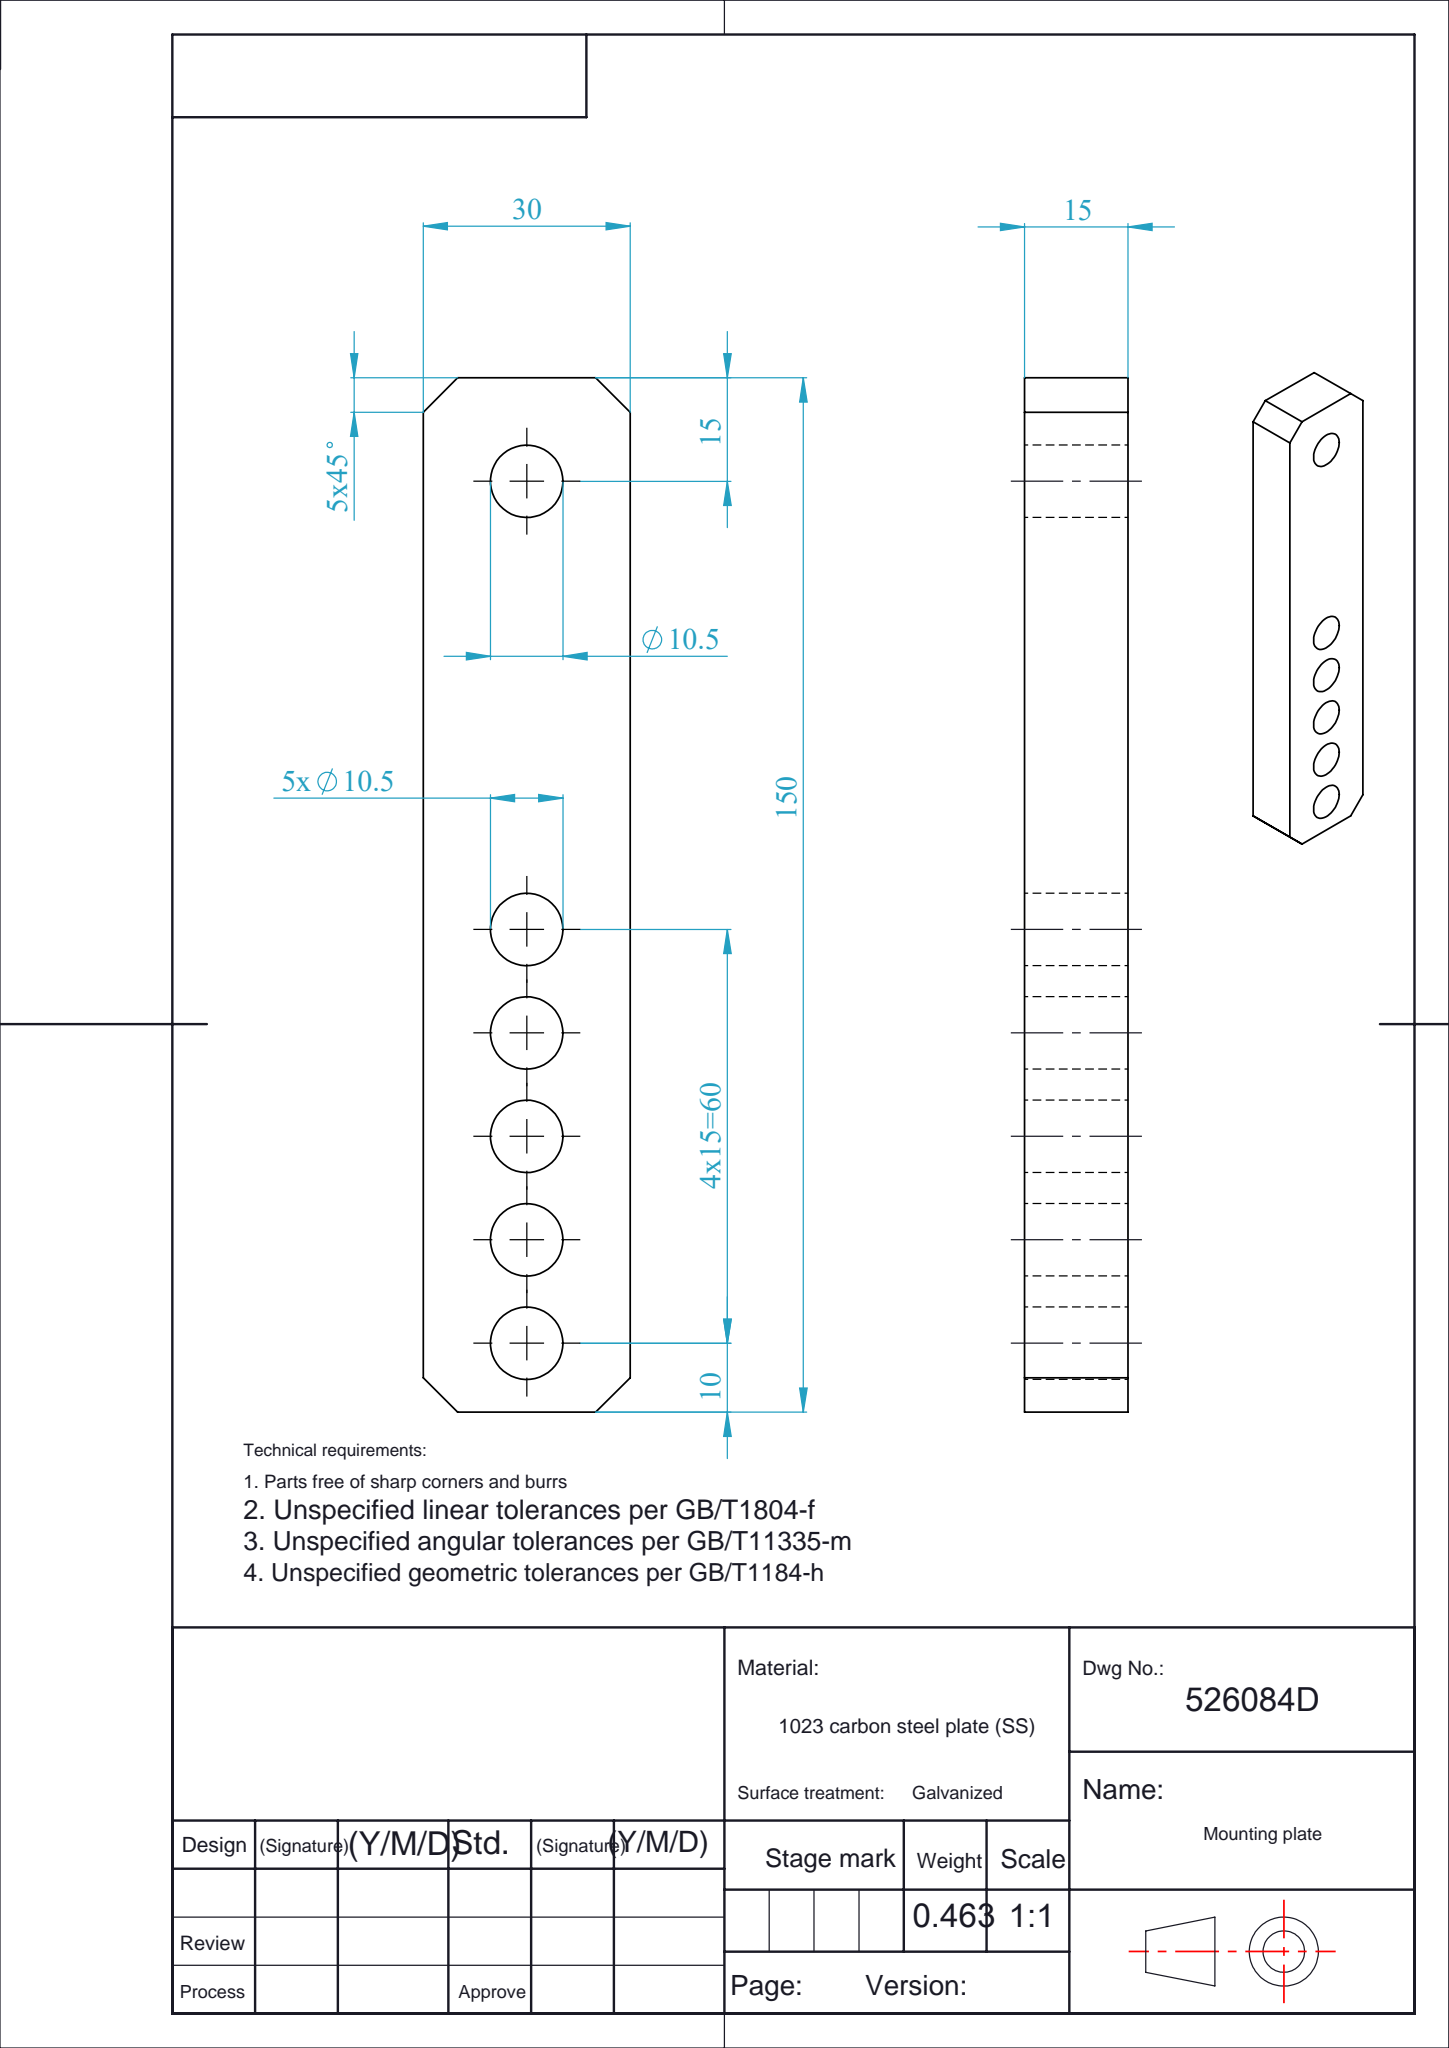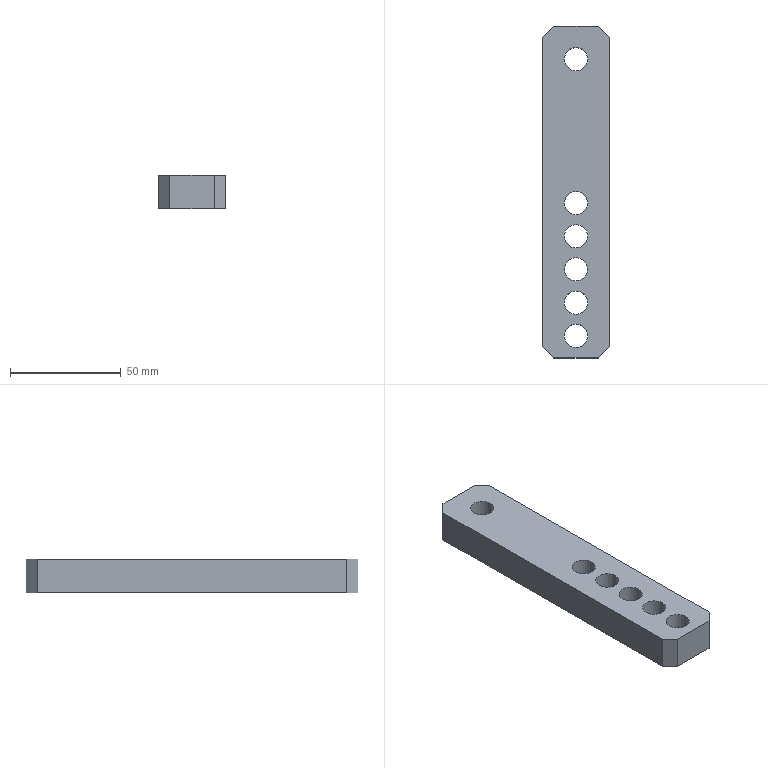Part | SolidWorks | features Chamfer 1, Extrusion 1, ICE 1 | 1 solid | 22 faces | box 30 x 150 x 15 mm | volume 58957 mm3 | cylinder 12 | plane 10 | commonest cylinder face diameters 10.5 x12
STEP:
#1=CARTESIAN_POINT('',(-5.25,60.,0.));
#2=VERTEX_POINT('',#1);
#3=CARTESIAN_POINT('',(5.25,60.,0.));
#4=VERTEX_POINT('',#3);
#5=CARTESIAN_POINT('',(0.,60.,0.));
#6=DIRECTION('',(0.,0.,1.));
#7=DIRECTION('',(1.,0.,0.));
#8=AXIS2_PLACEMENT_3D('',#5,#6,#7);
#9=CIRCLE('',#8,5.25);
#10=EDGE_CURVE('',#2,#4,#9,.T.);
#11=ORIENTED_EDGE('',*,*,#10,.F.);
#12=CARTESIAN_POINT('',(-5.25,60.,15.));
#13=VERTEX_POINT('',#12);
#14=CARTESIAN_POINT('',(-5.25,60.,-28.));
#15=DIRECTION('',(0.,0.,1.));
#16=VECTOR('',#15,1000.);
#17=LINE('',#14,#16);
#18=EDGE_CURVE('',#2,#13,#17,.T.);
#19=ORIENTED_EDGE('',*,*,#18,.T.);
#20=CARTESIAN_POINT('',(5.25,60.,15.));
#21=VERTEX_POINT('',#20);
#22=CARTESIAN_POINT('',(0.,60.,15.));
#23=DIRECTION('',(0.,0.,1.));
#24=DIRECTION('',(1.,0.,0.));
#25=AXIS2_PLACEMENT_3D('',#22,#23,#24);
#26=CIRCLE('',#25,5.25);
#27=EDGE_CURVE('',#13,#21,#26,.T.);
#28=ORIENTED_EDGE('',*,*,#27,.T.);
#29=CARTESIAN_POINT('',(5.25,60.,-28.));
#30=DIRECTION('',(0.,0.,1.));
#31=VECTOR('',#30,1000.);
#32=LINE('',#29,#31);
#33=EDGE_CURVE('',#4,#21,#32,.T.);
#34=ORIENTED_EDGE('',*,*,#33,.F.);
#35=EDGE_LOOP('',(#11,#19,#28,#34));
#36=FACE_OUTER_BOUND('',#35,.T.);
#37=CARTESIAN_POINT('',(0.,60.,-28.));
#38=DIRECTION('',(0.,0.,1.));
#39=DIRECTION('',(1.,0.,0.));
#40=AXIS2_PLACEMENT_3D('',#37,#38,#39);
#41=CYLINDRICAL_SURFACE('',#40,5.25);
#42=ADVANCED_FACE('',(#36),#41,.F.);
#43=CARTESIAN_POINT('',(-5.25,-5.,0.));
#44=VERTEX_POINT('',#43);
#45=CARTESIAN_POINT('',(5.25,-5.,0.));
#46=VERTEX_POINT('',#45);
#47=CARTESIAN_POINT('',(0.,-5.,0.));
#48=DIRECTION('',(0.,0.,1.));
#49=DIRECTION('',(1.,0.,0.));
#50=AXIS2_PLACEMENT_3D('',#47,#48,#49);
#51=CIRCLE('',#50,5.25);
#52=EDGE_CURVE('',#44,#46,#51,.T.);
#53=ORIENTED_EDGE('',*,*,#52,.F.);
#54=CARTESIAN_POINT('',(-5.25,-5.,15.));
#55=VERTEX_POINT('',#54);
#56=CARTESIAN_POINT('',(-5.25,-5.,-28.));
#57=DIRECTION('',(0.,0.,1.));
#58=VECTOR('',#57,1000.);
#59=LINE('',#56,#58);
#60=EDGE_CURVE('',#44,#55,#59,.T.);
#61=ORIENTED_EDGE('',*,*,#60,.T.);
#62=CARTESIAN_POINT('',(5.25,-5.,15.));
#63=VERTEX_POINT('',#62);
#64=CARTESIAN_POINT('',(0.,-5.,15.));
#65=DIRECTION('',(0.,0.,1.));
#66=DIRECTION('',(1.,0.,0.));
#67=AXIS2_PLACEMENT_3D('',#64,#65,#66);
#68=CIRCLE('',#67,5.25);
#69=EDGE_CURVE('',#55,#63,#68,.T.);
#70=ORIENTED_EDGE('',*,*,#69,.T.);
#71=CARTESIAN_POINT('',(5.25,-5.,-28.));
#72=DIRECTION('',(0.,0.,1.));
#73=VECTOR('',#72,1000.);
#74=LINE('',#71,#73);
#75=EDGE_CURVE('',#46,#63,#74,.T.);
#76=ORIENTED_EDGE('',*,*,#75,.F.);
#77=EDGE_LOOP('',(#53,#61,#70,#76));
#78=FACE_OUTER_BOUND('',#77,.T.);
#79=CARTESIAN_POINT('',(0.,-5.,-28.));
#80=DIRECTION('',(0.,0.,1.));
#81=DIRECTION('',(1.,0.,0.));
#82=AXIS2_PLACEMENT_3D('',#79,#80,#81);
#83=CYLINDRICAL_SURFACE('',#82,5.25);
#84=ADVANCED_FACE('',(#78),#83,.F.);
#85=CARTESIAN_POINT('',(-5.25,-20.,0.));
#86=VERTEX_POINT('',#85);
#87=CARTESIAN_POINT('',(5.25,-20.,0.));
#88=VERTEX_POINT('',#87);
#89=CARTESIAN_POINT('',(0.,-20.,0.));
#90=DIRECTION('',(0.,0.,1.));
#91=DIRECTION('',(1.,0.,0.));
#92=AXIS2_PLACEMENT_3D('',#89,#90,#91);
#93=CIRCLE('',#92,5.25);
#94=EDGE_CURVE('',#86,#88,#93,.T.);
#95=ORIENTED_EDGE('',*,*,#94,.F.);
#96=CARTESIAN_POINT('',(-5.25,-20.,15.));
#97=VERTEX_POINT('',#96);
#98=CARTESIAN_POINT('',(-5.25,-20.,-28.));
#99=DIRECTION('',(0.,0.,1.));
#100=VECTOR('',#99,1000.);
#101=LINE('',#98,#100);
#102=EDGE_CURVE('',#86,#97,#101,.T.);
#103=ORIENTED_EDGE('',*,*,#102,.T.);
#104=CARTESIAN_POINT('',(5.25,-20.,15.));
#105=VERTEX_POINT('',#104);
#106=CARTESIAN_POINT('',(0.,-20.,15.));
#107=DIRECTION('',(0.,0.,1.));
#108=DIRECTION('',(1.,0.,0.));
#109=AXIS2_PLACEMENT_3D('',#106,#107,#108);
#110=CIRCLE('',#109,5.25);
#111=EDGE_CURVE('',#97,#105,#110,.T.);
#112=ORIENTED_EDGE('',*,*,#111,.T.);
#113=CARTESIAN_POINT('',(5.25,-20.,-28.));
#114=DIRECTION('',(0.,0.,1.));
#115=VECTOR('',#114,1000.);
#116=LINE('',#113,#115);
#117=EDGE_CURVE('',#88,#105,#116,.T.);
#118=ORIENTED_EDGE('',*,*,#117,.F.);
#119=EDGE_LOOP('',(#95,#103,#112,#118));
#120=FACE_OUTER_BOUND('',#119,.T.);
#121=CARTESIAN_POINT('',(0.,-20.,-28.));
#122=DIRECTION('',(0.,0.,1.));
#123=DIRECTION('',(1.,0.,0.));
#124=AXIS2_PLACEMENT_3D('',#121,#122,#123);
#125=CYLINDRICAL_SURFACE('',#124,5.25);
#126=ADVANCED_FACE('',(#120),#125,.F.);
#127=CARTESIAN_POINT('',(-5.25,-35.,0.));
#128=VERTEX_POINT('',#127);
#129=CARTESIAN_POINT('',(5.25,-35.,0.));
#130=VERTEX_POINT('',#129);
#131=CARTESIAN_POINT('',(0.,-35.,0.));
#132=DIRECTION('',(0.,0.,1.));
#133=DIRECTION('',(1.,0.,0.));
#134=AXIS2_PLACEMENT_3D('',#131,#132,#133);
#135=CIRCLE('',#134,5.25);
#136=EDGE_CURVE('',#128,#130,#135,.T.);
#137=ORIENTED_EDGE('',*,*,#136,.F.);
#138=CARTESIAN_POINT('',(-5.25,-35.,15.));
#139=VERTEX_POINT('',#138);
#140=CARTESIAN_POINT('',(-5.25,-35.,-28.));
#141=DIRECTION('',(0.,0.,1.));
#142=VECTOR('',#141,1000.);
#143=LINE('',#140,#142);
#144=EDGE_CURVE('',#128,#139,#143,.T.);
#145=ORIENTED_EDGE('',*,*,#144,.T.);
#146=CARTESIAN_POINT('',(5.25,-35.,15.));
#147=VERTEX_POINT('',#146);
#148=CARTESIAN_POINT('',(0.,-35.,15.));
#149=DIRECTION('',(0.,0.,1.));
#150=DIRECTION('',(1.,0.,0.));
#151=AXIS2_PLACEMENT_3D('',#148,#149,#150);
#152=CIRCLE('',#151,5.25);
#153=EDGE_CURVE('',#139,#147,#152,.T.);
#154=ORIENTED_EDGE('',*,*,#153,.T.);
#155=CARTESIAN_POINT('',(5.25,-35.,-28.));
#156=DIRECTION('',(0.,0.,1.));
#157=VECTOR('',#156,1000.);
#158=LINE('',#155,#157);
#159=EDGE_CURVE('',#130,#147,#158,.T.);
#160=ORIENTED_EDGE('',*,*,#159,.F.);
#161=EDGE_LOOP('',(#137,#145,#154,#160));
#162=FACE_OUTER_BOUND('',#161,.T.);
#163=CARTESIAN_POINT('',(0.,-35.,-28.));
#164=DIRECTION('',(0.,0.,1.));
#165=DIRECTION('',(1.,0.,0.));
#166=AXIS2_PLACEMENT_3D('',#163,#164,#165);
#167=CYLINDRICAL_SURFACE('',#166,5.25);
#168=ADVANCED_FACE('',(#162),#167,.F.);
#169=CARTESIAN_POINT('',(-5.25,-50.,0.));
#170=VERTEX_POINT('',#169);
#171=CARTESIAN_POINT('',(5.25,-50.,0.));
#172=VERTEX_POINT('',#171);
#173=CARTESIAN_POINT('',(0.,-50.,0.));
#174=DIRECTION('',(0.,0.,1.));
#175=DIRECTION('',(1.,0.,0.));
#176=AXIS2_PLACEMENT_3D('',#173,#174,#175);
#177=CIRCLE('',#176,5.25);
#178=EDGE_CURVE('',#170,#172,#177,.T.);
#179=ORIENTED_EDGE('',*,*,#178,.F.);
#180=CARTESIAN_POINT('',(-5.25,-50.,15.));
#181=VERTEX_POINT('',#180);
#182=CARTESIAN_POINT('',(-5.25,-50.,-28.));
#183=DIRECTION('',(0.,0.,1.));
#184=VECTOR('',#183,1000.);
#185=LINE('',#182,#184);
#186=EDGE_CURVE('',#170,#181,#185,.T.);
#187=ORIENTED_EDGE('',*,*,#186,.T.);
#188=CARTESIAN_POINT('',(5.25,-50.,15.));
#189=VERTEX_POINT('',#188);
#190=CARTESIAN_POINT('',(0.,-50.,15.));
#191=DIRECTION('',(0.,0.,1.));
#192=DIRECTION('',(1.,0.,0.));
#193=AXIS2_PLACEMENT_3D('',#190,#191,#192);
#194=CIRCLE('',#193,5.25);
#195=EDGE_CURVE('',#181,#189,#194,.T.);
#196=ORIENTED_EDGE('',*,*,#195,.T.);
#197=CARTESIAN_POINT('',(5.25,-50.,-28.));
#198=DIRECTION('',(0.,0.,1.));
#199=VECTOR('',#198,1000.);
#200=LINE('',#197,#199);
#201=EDGE_CURVE('',#172,#189,#200,.T.);
#202=ORIENTED_EDGE('',*,*,#201,.F.);
#203=EDGE_LOOP('',(#179,#187,#196,#202));
#204=FACE_OUTER_BOUND('',#203,.T.);
#205=CARTESIAN_POINT('',(0.,-50.,-28.));
#206=DIRECTION('',(0.,0.,1.));
#207=DIRECTION('',(1.,0.,0.));
#208=AXIS2_PLACEMENT_3D('',#205,#206,#207);
#209=CYLINDRICAL_SURFACE('',#208,5.25);
#210=ADVANCED_FACE('',(#204),#209,.F.);
#211=CARTESIAN_POINT('',(-5.25,-65.,0.));
#212=VERTEX_POINT('',#211);
#213=CARTESIAN_POINT('',(5.25,-65.,0.));
#214=VERTEX_POINT('',#213);
#215=CARTESIAN_POINT('',(0.,-65.,0.));
#216=DIRECTION('',(0.,0.,1.));
#217=DIRECTION('',(1.,0.,0.));
#218=AXIS2_PLACEMENT_3D('',#215,#216,#217);
#219=CIRCLE('',#218,5.25);
#220=EDGE_CURVE('',#212,#214,#219,.T.);
#221=ORIENTED_EDGE('',*,*,#220,.F.);
#222=CARTESIAN_POINT('',(-5.25,-65.,15.));
#223=VERTEX_POINT('',#222);
#224=CARTESIAN_POINT('',(-5.25,-65.,-28.));
#225=DIRECTION('',(0.,0.,1.));
#226=VECTOR('',#225,1000.);
#227=LINE('',#224,#226);
#228=EDGE_CURVE('',#212,#223,#227,.T.);
#229=ORIENTED_EDGE('',*,*,#228,.T.);
#230=CARTESIAN_POINT('',(5.25,-65.,15.));
#231=VERTEX_POINT('',#230);
#232=CARTESIAN_POINT('',(0.,-65.,15.));
#233=DIRECTION('',(0.,0.,1.));
#234=DIRECTION('',(1.,0.,0.));
#235=AXIS2_PLACEMENT_3D('',#232,#233,#234);
#236=CIRCLE('',#235,5.25);
#237=EDGE_CURVE('',#223,#231,#236,.T.);
#238=ORIENTED_EDGE('',*,*,#237,.T.);
#239=CARTESIAN_POINT('',(5.25,-65.,-28.));
#240=DIRECTION('',(0.,0.,1.));
#241=VECTOR('',#240,1000.);
#242=LINE('',#239,#241);
#243=EDGE_CURVE('',#214,#231,#242,.T.);
#244=ORIENTED_EDGE('',*,*,#243,.F.);
#245=EDGE_LOOP('',(#221,#229,#238,#244));
#246=FACE_OUTER_BOUND('',#245,.T.);
#247=CARTESIAN_POINT('',(0.,-65.,-28.));
#248=DIRECTION('',(0.,0.,1.));
#249=DIRECTION('',(1.,0.,0.));
#250=AXIS2_PLACEMENT_3D('',#247,#248,#249);
#251=CYLINDRICAL_SURFACE('',#250,5.25);
#252=ADVANCED_FACE('',(#246),#251,.F.);
#253=CARTESIAN_POINT('',(15.,-70.,15.));
#254=VERTEX_POINT('',#253);
#255=CARTESIAN_POINT('',(15.,70.,15.));
#256=VERTEX_POINT('',#255);
#257=CARTESIAN_POINT('',(15.,75.,15.));
#258=DIRECTION('',(0.,1.,0.));
#259=VECTOR('',#258,1000.);
#260=LINE('',#257,#259);
#261=EDGE_CURVE('',#254,#256,#260,.T.);
#262=ORIENTED_EDGE('',*,*,#261,.F.);
#263=CARTESIAN_POINT('',(15.,-70.,0.));
#264=VERTEX_POINT('',#263);
#265=CARTESIAN_POINT('',(15.,-70.,15.));
#266=DIRECTION('',(0.,0.,-1.));
#267=VECTOR('',#266,1000.);
#268=LINE('',#265,#267);
#269=EDGE_CURVE('',#254,#264,#268,.T.);
#270=ORIENTED_EDGE('',*,*,#269,.T.);
#271=CARTESIAN_POINT('',(15.,70.,0.));
#272=VERTEX_POINT('',#271);
#273=CARTESIAN_POINT('',(15.,75.,0.));
#274=DIRECTION('',(0.,1.,0.));
#275=VECTOR('',#274,1000.);
#276=LINE('',#273,#275);
#277=EDGE_CURVE('',#264,#272,#276,.T.);
#278=ORIENTED_EDGE('',*,*,#277,.T.);
#279=CARTESIAN_POINT('',(15.,70.,15.));
#280=DIRECTION('',(0.,0.,1.));
#281=VECTOR('',#280,1000.);
#282=LINE('',#279,#281);
#283=EDGE_CURVE('',#272,#256,#282,.T.);
#284=ORIENTED_EDGE('',*,*,#283,.T.);
#285=EDGE_LOOP('',(#262,#270,#278,#284));
#286=FACE_OUTER_BOUND('',#285,.T.);
#287=CARTESIAN_POINT('',(15.,75.,15.));
#288=DIRECTION('',(-1.,0.,0.));
#289=DIRECTION('',(0.,-1.,0.));
#290=AXIS2_PLACEMENT_3D('',#287,#288,#289);
#291=PLANE('',#290);
#292=ADVANCED_FACE('',(#286),#291,.F.);
#293=CARTESIAN_POINT('',(10.,75.,0.));
#294=VERTEX_POINT('',#293);
#295=CARTESIAN_POINT('',(-10.,75.,0.));
#296=VERTEX_POINT('',#295);
#297=CARTESIAN_POINT('',(-15.,75.,0.));
#298=DIRECTION('',(-1.,0.,0.));
#299=VECTOR('',#298,1000.);
#300=LINE('',#297,#299);
#301=EDGE_CURVE('',#294,#296,#300,.T.);
#302=ORIENTED_EDGE('',*,*,#301,.T.);
#303=CARTESIAN_POINT('',(-10.,75.,15.));
#304=VERTEX_POINT('',#303);
#305=CARTESIAN_POINT('',(-10.,75.,15.));
#306=DIRECTION('',(0.,0.,1.));
#307=VECTOR('',#306,1000.);
#308=LINE('',#305,#307);
#309=EDGE_CURVE('',#296,#304,#308,.T.);
#310=ORIENTED_EDGE('',*,*,#309,.T.);
#311=CARTESIAN_POINT('',(10.,75.,15.));
#312=VERTEX_POINT('',#311);
#313=CARTESIAN_POINT('',(-15.,75.,15.));
#314=DIRECTION('',(-1.,0.,0.));
#315=VECTOR('',#314,1000.);
#316=LINE('',#313,#315);
#317=EDGE_CURVE('',#312,#304,#316,.T.);
#318=ORIENTED_EDGE('',*,*,#317,.F.);
#319=CARTESIAN_POINT('',(10.,75.,15.));
#320=DIRECTION('',(0.,0.,-1.));
#321=VECTOR('',#320,1000.);
#322=LINE('',#319,#321);
#323=EDGE_CURVE('',#312,#294,#322,.T.);
#324=ORIENTED_EDGE('',*,*,#323,.T.);
#325=EDGE_LOOP('',(#302,#310,#318,#324));
#326=FACE_OUTER_BOUND('',#325,.T.);
#327=CARTESIAN_POINT('',(-15.,75.,15.));
#328=DIRECTION('',(0.,-1.,0.));
#329=DIRECTION('',(0.,0.,-1.));
#330=AXIS2_PLACEMENT_3D('',#327,#328,#329);
#331=PLANE('',#330);
#332=ADVANCED_FACE('',(#326),#331,.F.);
#333=CARTESIAN_POINT('',(-15.,70.,0.));
#334=VERTEX_POINT('',#333);
#335=CARTESIAN_POINT('',(-15.,-70.,0.));
#336=VERTEX_POINT('',#335);
#337=CARTESIAN_POINT('',(-15.,75.,0.));
#338=DIRECTION('',(0.,-1.,0.));
#339=VECTOR('',#338,1000.);
#340=LINE('',#337,#339);
#341=EDGE_CURVE('',#334,#336,#340,.T.);
#342=ORIENTED_EDGE('',*,*,#341,.T.);
#343=CARTESIAN_POINT('',(-15.,-70.,15.));
#344=VERTEX_POINT('',#343);
#345=CARTESIAN_POINT('',(-15.,-70.,15.));
#346=DIRECTION('',(0.,0.,1.));
#347=VECTOR('',#346,1000.);
#348=LINE('',#345,#347);
#349=EDGE_CURVE('',#336,#344,#348,.T.);
#350=ORIENTED_EDGE('',*,*,#349,.T.);
#351=CARTESIAN_POINT('',(-15.,70.,15.));
#352=VERTEX_POINT('',#351);
#353=CARTESIAN_POINT('',(-15.,75.,15.));
#354=DIRECTION('',(0.,-1.,0.));
#355=VECTOR('',#354,1000.);
#356=LINE('',#353,#355);
#357=EDGE_CURVE('',#352,#344,#356,.T.);
#358=ORIENTED_EDGE('',*,*,#357,.F.);
#359=CARTESIAN_POINT('',(-15.,70.,15.));
#360=DIRECTION('',(0.,0.,-1.));
#361=VECTOR('',#360,1000.);
#362=LINE('',#359,#361);
#363=EDGE_CURVE('',#352,#334,#362,.T.);
#364=ORIENTED_EDGE('',*,*,#363,.T.);
#365=EDGE_LOOP('',(#342,#350,#358,#364));
#366=FACE_OUTER_BOUND('',#365,.T.);
#367=CARTESIAN_POINT('',(-15.,75.,15.));
#368=DIRECTION('',(1.,0.,0.));
#369=DIRECTION('',(0.,1.,0.));
#370=AXIS2_PLACEMENT_3D('',#367,#368,#369);
#371=PLANE('',#370);
#372=ADVANCED_FACE('',(#366),#371,.F.);
#373=CARTESIAN_POINT('',(-10.,-75.,15.));
#374=VERTEX_POINT('',#373);
#375=CARTESIAN_POINT('',(10.,-75.,15.));
#376=VERTEX_POINT('',#375);
#377=CARTESIAN_POINT('',(-15.,-75.,15.));
#378=DIRECTION('',(1.,0.,0.));
#379=VECTOR('',#378,1000.);
#380=LINE('',#377,#379);
#381=EDGE_CURVE('',#374,#376,#380,.T.);
#382=ORIENTED_EDGE('',*,*,#381,.F.);
#383=CARTESIAN_POINT('',(-10.,-75.,0.));
#384=VERTEX_POINT('',#383);
#385=CARTESIAN_POINT('',(-10.,-75.,15.));
#386=DIRECTION('',(0.,0.,-1.));
#387=VECTOR('',#386,1000.);
#388=LINE('',#385,#387);
#389=EDGE_CURVE('',#374,#384,#388,.T.);
#390=ORIENTED_EDGE('',*,*,#389,.T.);
#391=CARTESIAN_POINT('',(10.,-75.,0.));
#392=VERTEX_POINT('',#391);
#393=CARTESIAN_POINT('',(-15.,-75.,0.));
#394=DIRECTION('',(1.,0.,0.));
#395=VECTOR('',#394,1000.);
#396=LINE('',#393,#395);
#397=EDGE_CURVE('',#384,#392,#396,.T.);
#398=ORIENTED_EDGE('',*,*,#397,.T.);
#399=CARTESIAN_POINT('',(10.,-75.,15.));
#400=DIRECTION('',(0.,0.,1.));
#401=VECTOR('',#400,1000.);
#402=LINE('',#399,#401);
#403=EDGE_CURVE('',#392,#376,#402,.T.);
#404=ORIENTED_EDGE('',*,*,#403,.T.);
#405=EDGE_LOOP('',(#382,#390,#398,#404));
#406=FACE_OUTER_BOUND('',#405,.T.);
#407=CARTESIAN_POINT('',(-15.,-75.,15.));
#408=DIRECTION('',(0.,1.,0.));
#409=DIRECTION('',(0.,0.,1.));
#410=AXIS2_PLACEMENT_3D('',#407,#408,#409);
#411=PLANE('',#410);
#412=ADVANCED_FACE('',(#406),#411,.F.);
#413=CARTESIAN_POINT('',(0.,60.,15.));
#414=DIRECTION('',(0.,0.,1.));
#415=DIRECTION('',(1.,0.,0.));
#416=AXIS2_PLACEMENT_3D('',#413,#414,#415);
#417=CIRCLE('',#416,5.25);
#418=EDGE_CURVE('',#21,#13,#417,.T.);
#419=ORIENTED_EDGE('',*,*,#418,.F.);
#420=ORIENTED_EDGE('',*,*,#27,.F.);
#421=EDGE_LOOP('',(#419,#420));
#422=FACE_BOUND('',#421,.T.);
#423=CARTESIAN_POINT('',(0.,-5.,15.));
#424=DIRECTION('',(0.,0.,1.));
#425=DIRECTION('',(1.,0.,0.));
#426=AXIS2_PLACEMENT_3D('',#423,#424,#425);
#427=CIRCLE('',#426,5.25);
#428=EDGE_CURVE('',#63,#55,#427,.T.);
#429=ORIENTED_EDGE('',*,*,#428,.F.);
#430=ORIENTED_EDGE('',*,*,#69,.F.);
#431=EDGE_LOOP('',(#429,#430));
#432=FACE_BOUND('',#431,.T.);
#433=CARTESIAN_POINT('',(0.,-20.,15.));
#434=DIRECTION('',(0.,0.,1.));
#435=DIRECTION('',(1.,0.,0.));
#436=AXIS2_PLACEMENT_3D('',#433,#434,#435);
#437=CIRCLE('',#436,5.25);
#438=EDGE_CURVE('',#105,#97,#437,.T.);
#439=ORIENTED_EDGE('',*,*,#438,.F.);
#440=ORIENTED_EDGE('',*,*,#111,.F.);
#441=EDGE_LOOP('',(#439,#440));
#442=FACE_BOUND('',#441,.T.);
#443=CARTESIAN_POINT('',(0.,-35.,15.));
#444=DIRECTION('',(0.,0.,1.));
#445=DIRECTION('',(1.,0.,0.));
#446=AXIS2_PLACEMENT_3D('',#443,#444,#445);
#447=CIRCLE('',#446,5.25);
#448=EDGE_CURVE('',#147,#139,#447,.T.);
#449=ORIENTED_EDGE('',*,*,#448,.F.);
#450=ORIENTED_EDGE('',*,*,#153,.F.);
#451=EDGE_LOOP('',(#449,#450));
#452=FACE_BOUND('',#451,.T.);
#453=CARTESIAN_POINT('',(0.,-50.,15.));
#454=DIRECTION('',(0.,0.,1.));
#455=DIRECTION('',(1.,0.,0.));
#456=AXIS2_PLACEMENT_3D('',#453,#454,#455);
#457=CIRCLE('',#456,5.25);
#458=EDGE_CURVE('',#189,#181,#457,.T.);
#459=ORIENTED_EDGE('',*,*,#458,.F.);
#460=ORIENTED_EDGE('',*,*,#195,.F.);
#461=EDGE_LOOP('',(#459,#460));
#462=FACE_BOUND('',#461,.T.);
#463=CARTESIAN_POINT('',(0.,-65.,15.));
#464=DIRECTION('',(0.,0.,1.));
#465=DIRECTION('',(1.,0.,0.));
#466=AXIS2_PLACEMENT_3D('',#463,#464,#465);
#467=CIRCLE('',#466,5.25);
#468=EDGE_CURVE('',#231,#223,#467,.T.);
#469=ORIENTED_EDGE('',*,*,#468,.F.);
#470=ORIENTED_EDGE('',*,*,#237,.F.);
#471=EDGE_LOOP('',(#469,#470));
#472=FACE_BOUND('',#471,.T.);
#473=ORIENTED_EDGE('',*,*,#357,.T.);
#474=CARTESIAN_POINT('',(-42.5,-42.5,15.));
#475=DIRECTION('',(0.7071,-0.7071,0.));
#476=VECTOR('',#475,1000.);
#477=LINE('',#474,#476);
#478=EDGE_CURVE('',#344,#374,#477,.T.);
#479=ORIENTED_EDGE('',*,*,#478,.T.);
#480=ORIENTED_EDGE('',*,*,#381,.T.);
#481=CARTESIAN_POINT('',(42.5,-42.5,15.));
#482=DIRECTION('',(0.7071,0.7071,0.));
#483=VECTOR('',#482,1000.);
#484=LINE('',#481,#483);
#485=EDGE_CURVE('',#376,#254,#484,.T.);
#486=ORIENTED_EDGE('',*,*,#485,.T.);
#487=ORIENTED_EDGE('',*,*,#261,.T.);
#488=CARTESIAN_POINT('',(42.5,42.5,15.));
#489=DIRECTION('',(-0.7071,0.7071,0.));
#490=VECTOR('',#489,1000.);
#491=LINE('',#488,#490);
#492=EDGE_CURVE('',#256,#312,#491,.T.);
#493=ORIENTED_EDGE('',*,*,#492,.T.);
#494=ORIENTED_EDGE('',*,*,#317,.T.);
#495=CARTESIAN_POINT('',(-42.5,42.5,15.));
#496=DIRECTION('',(-0.7071,-0.7071,0.));
#497=VECTOR('',#496,1000.);
#498=LINE('',#495,#497);
#499=EDGE_CURVE('',#304,#352,#498,.T.);
#500=ORIENTED_EDGE('',*,*,#499,.T.);
#501=EDGE_LOOP('',(#473,#479,#480,#486,#487,#493,#494,#500));
#502=FACE_OUTER_BOUND('',#501,.T.);
#503=CARTESIAN_POINT('',(0.,0.,15.));
#504=DIRECTION('',(0.,0.,1.));
#505=DIRECTION('',(1.,0.,0.));
#506=AXIS2_PLACEMENT_3D('',#503,#504,#505);
#507=PLANE('',#506);
#508=ADVANCED_FACE('',(#422,#432,#442,#452,#462,#472,#502),#507,.T.);
#509=CARTESIAN_POINT('',(0.,60.,0.));
#510=DIRECTION('',(0.,0.,1.));
#511=DIRECTION('',(1.,0.,0.));
#512=AXIS2_PLACEMENT_3D('',#509,#510,#511);
#513=CIRCLE('',#512,5.25);
#514=EDGE_CURVE('',#4,#2,#513,.T.);
#515=ORIENTED_EDGE('',*,*,#514,.T.);
#516=ORIENTED_EDGE('',*,*,#10,.T.);
#517=EDGE_LOOP('',(#515,#516));
#518=FACE_BOUND('',#517,.T.);
#519=CARTESIAN_POINT('',(0.,-5.,0.));
#520=DIRECTION('',(0.,0.,1.));
#521=DIRECTION('',(1.,0.,0.));
#522=AXIS2_PLACEMENT_3D('',#519,#520,#521);
#523=CIRCLE('',#522,5.25);
#524=EDGE_CURVE('',#46,#44,#523,.T.);
#525=ORIENTED_EDGE('',*,*,#524,.T.);
#526=ORIENTED_EDGE('',*,*,#52,.T.);
#527=EDGE_LOOP('',(#525,#526));
#528=FACE_BOUND('',#527,.T.);
#529=CARTESIAN_POINT('',(0.,-20.,0.));
#530=DIRECTION('',(0.,0.,1.));
#531=DIRECTION('',(1.,0.,0.));
#532=AXIS2_PLACEMENT_3D('',#529,#530,#531);
#533=CIRCLE('',#532,5.25);
#534=EDGE_CURVE('',#88,#86,#533,.T.);
#535=ORIENTED_EDGE('',*,*,#534,.T.);
#536=ORIENTED_EDGE('',*,*,#94,.T.);
#537=EDGE_LOOP('',(#535,#536));
#538=FACE_BOUND('',#537,.T.);
#539=CARTESIAN_POINT('',(0.,-35.,0.));
#540=DIRECTION('',(0.,0.,1.));
#541=DIRECTION('',(1.,0.,0.));
#542=AXIS2_PLACEMENT_3D('',#539,#540,#541);
#543=CIRCLE('',#542,5.25);
#544=EDGE_CURVE('',#130,#128,#543,.T.);
#545=ORIENTED_EDGE('',*,*,#544,.T.);
#546=ORIENTED_EDGE('',*,*,#136,.T.);
#547=EDGE_LOOP('',(#545,#546));
#548=FACE_BOUND('',#547,.T.);
#549=CARTESIAN_POINT('',(0.,-50.,0.));
#550=DIRECTION('',(0.,0.,1.));
#551=DIRECTION('',(1.,0.,0.));
#552=AXIS2_PLACEMENT_3D('',#549,#550,#551);
#553=CIRCLE('',#552,5.25);
#554=EDGE_CURVE('',#172,#170,#553,.T.);
#555=ORIENTED_EDGE('',*,*,#554,.T.);
#556=ORIENTED_EDGE('',*,*,#178,.T.);
#557=EDGE_LOOP('',(#555,#556));
#558=FACE_BOUND('',#557,.T.);
#559=CARTESIAN_POINT('',(0.,-65.,0.));
#560=DIRECTION('',(0.,0.,1.));
#561=DIRECTION('',(1.,0.,0.));
#562=AXIS2_PLACEMENT_3D('',#559,#560,#561);
#563=CIRCLE('',#562,5.25);
#564=EDGE_CURVE('',#214,#212,#563,.T.);
#565=ORIENTED_EDGE('',*,*,#564,.T.);
#566=ORIENTED_EDGE('',*,*,#220,.T.);
#567=EDGE_LOOP('',(#565,#566));
#568=FACE_BOUND('',#567,.T.);
#569=ORIENTED_EDGE('',*,*,#397,.F.);
#570=CARTESIAN_POINT('',(-10.,-75.,0.));
#571=DIRECTION('',(-0.7071,0.7071,0.));
#572=VECTOR('',#571,1000.);
#573=LINE('',#570,#572);
#574=EDGE_CURVE('',#384,#336,#573,.T.);
#575=ORIENTED_EDGE('',*,*,#574,.T.);
#576=ORIENTED_EDGE('',*,*,#341,.F.);
#577=CARTESIAN_POINT('',(-15.,70.,0.));
#578=DIRECTION('',(0.7071,0.7071,0.));
#579=VECTOR('',#578,1000.);
#580=LINE('',#577,#579);
#581=EDGE_CURVE('',#334,#296,#580,.T.);
#582=ORIENTED_EDGE('',*,*,#581,.T.);
#583=ORIENTED_EDGE('',*,*,#301,.F.);
#584=CARTESIAN_POINT('',(10.,75.,0.));
#585=DIRECTION('',(0.7071,-0.7071,0.));
#586=VECTOR('',#585,1000.);
#587=LINE('',#584,#586);
#588=EDGE_CURVE('',#294,#272,#587,.T.);
#589=ORIENTED_EDGE('',*,*,#588,.T.);
#590=ORIENTED_EDGE('',*,*,#277,.F.);
#591=CARTESIAN_POINT('',(15.,-70.,0.));
#592=DIRECTION('',(-0.7071,-0.7071,0.));
#593=VECTOR('',#592,1000.);
#594=LINE('',#591,#593);
#595=EDGE_CURVE('',#264,#392,#594,.T.);
#596=ORIENTED_EDGE('',*,*,#595,.T.);
#597=EDGE_LOOP('',(#569,#575,#576,#582,#583,#589,#590,#596));
#598=FACE_OUTER_BOUND('',#597,.T.);
#599=CARTESIAN_POINT('',(0.,0.,0.));
#600=DIRECTION('',(0.,0.,1.));
#601=DIRECTION('',(1.,0.,0.));
#602=AXIS2_PLACEMENT_3D('',#599,#600,#601);
#603=PLANE('',#602);
#604=ADVANCED_FACE('',(#518,#528,#538,#548,#558,#568,#598),#603,.F.);
#605=ORIENTED_EDGE('',*,*,#478,.F.);
#606=ORIENTED_EDGE('',*,*,#349,.F.);
#607=ORIENTED_EDGE('',*,*,#574,.F.);
#608=ORIENTED_EDGE('',*,*,#389,.F.);
#609=EDGE_LOOP('',(#605,#606,#607,#608));
#610=FACE_OUTER_BOUND('',#609,.T.);
#611=CARTESIAN_POINT('',(-10.,-75.,15.));
#612=DIRECTION('',(0.7071,0.7071,0.));
#613=DIRECTION('',(0.,0.,-1.));
#614=AXIS2_PLACEMENT_3D('',#611,#612,#613);
#615=PLANE('',#614);
#616=ADVANCED_FACE('',(#610),#615,.F.);
#617=ORIENTED_EDGE('',*,*,#485,.F.);
#618=ORIENTED_EDGE('',*,*,#403,.F.);
#619=ORIENTED_EDGE('',*,*,#595,.F.);
#620=ORIENTED_EDGE('',*,*,#269,.F.);
#621=EDGE_LOOP('',(#617,#618,#619,#620));
#622=FACE_OUTER_BOUND('',#621,.T.);
#623=CARTESIAN_POINT('',(15.,-70.,15.));
#624=DIRECTION('',(-0.7071,0.7071,0.));
#625=DIRECTION('',(0.,0.,-1.));
#626=AXIS2_PLACEMENT_3D('',#623,#624,#625);
#627=PLANE('',#626);
#628=ADVANCED_FACE('',(#622),#627,.F.);
#629=ORIENTED_EDGE('',*,*,#499,.F.);
#630=ORIENTED_EDGE('',*,*,#309,.F.);
#631=ORIENTED_EDGE('',*,*,#581,.F.);
#632=ORIENTED_EDGE('',*,*,#363,.F.);
#633=EDGE_LOOP('',(#629,#630,#631,#632));
#634=FACE_OUTER_BOUND('',#633,.T.);
#635=CARTESIAN_POINT('',(-15.,70.,15.));
#636=DIRECTION('',(0.7071,-0.7071,0.));
#637=DIRECTION('',(0.,0.,-1.));
#638=AXIS2_PLACEMENT_3D('',#635,#636,#637);
#639=PLANE('',#638);
#640=ADVANCED_FACE('',(#634),#639,.F.);
#641=ORIENTED_EDGE('',*,*,#492,.F.);
#642=ORIENTED_EDGE('',*,*,#283,.F.);
#643=ORIENTED_EDGE('',*,*,#588,.F.);
#644=ORIENTED_EDGE('',*,*,#323,.F.);
#645=EDGE_LOOP('',(#641,#642,#643,#644));
#646=FACE_OUTER_BOUND('',#645,.T.);
#647=CARTESIAN_POINT('',(10.,75.,15.));
#648=DIRECTION('',(-0.7071,-0.7071,0.));
#649=DIRECTION('',(0.,0.,-1.));
#650=AXIS2_PLACEMENT_3D('',#647,#648,#649);
#651=PLANE('',#650);
#652=ADVANCED_FACE('',(#646),#651,.F.);
#653=ORIENTED_EDGE('',*,*,#228,.F.);
#654=ORIENTED_EDGE('',*,*,#564,.F.);
#655=ORIENTED_EDGE('',*,*,#243,.T.);
#656=ORIENTED_EDGE('',*,*,#468,.T.);
#657=EDGE_LOOP('',(#653,#654,#655,#656));
#658=FACE_OUTER_BOUND('',#657,.T.);
#659=CARTESIAN_POINT('',(0.,-65.,-28.));
#660=DIRECTION('',(0.,0.,1.));
#661=DIRECTION('',(1.,0.,0.));
#662=AXIS2_PLACEMENT_3D('',#659,#660,#661);
#663=CYLINDRICAL_SURFACE('',#662,5.25);
#664=ADVANCED_FACE('',(#658),#663,.F.);
#665=ORIENTED_EDGE('',*,*,#186,.F.);
#666=ORIENTED_EDGE('',*,*,#554,.F.);
#667=ORIENTED_EDGE('',*,*,#201,.T.);
#668=ORIENTED_EDGE('',*,*,#458,.T.);
#669=EDGE_LOOP('',(#665,#666,#667,#668));
#670=FACE_OUTER_BOUND('',#669,.T.);
#671=CARTESIAN_POINT('',(0.,-50.,-28.));
#672=DIRECTION('',(0.,0.,1.));
#673=DIRECTION('',(1.,0.,0.));
#674=AXIS2_PLACEMENT_3D('',#671,#672,#673);
#675=CYLINDRICAL_SURFACE('',#674,5.25);
#676=ADVANCED_FACE('',(#670),#675,.F.);
#677=ORIENTED_EDGE('',*,*,#144,.F.);
#678=ORIENTED_EDGE('',*,*,#544,.F.);
#679=ORIENTED_EDGE('',*,*,#159,.T.);
#680=ORIENTED_EDGE('',*,*,#448,.T.);
#681=EDGE_LOOP('',(#677,#678,#679,#680));
#682=FACE_OUTER_BOUND('',#681,.T.);
#683=CARTESIAN_POINT('',(0.,-35.,-28.));
#684=DIRECTION('',(0.,0.,1.));
#685=DIRECTION('',(1.,0.,0.));
#686=AXIS2_PLACEMENT_3D('',#683,#684,#685);
#687=CYLINDRICAL_SURFACE('',#686,5.25);
#688=ADVANCED_FACE('',(#682),#687,.F.);
#689=ORIENTED_EDGE('',*,*,#102,.F.);
#690=ORIENTED_EDGE('',*,*,#534,.F.);
#691=ORIENTED_EDGE('',*,*,#117,.T.);
#692=ORIENTED_EDGE('',*,*,#438,.T.);
#693=EDGE_LOOP('',(#689,#690,#691,#692));
#694=FACE_OUTER_BOUND('',#693,.T.);
#695=CARTESIAN_POINT('',(0.,-20.,-28.));
#696=DIRECTION('',(0.,0.,1.));
#697=DIRECTION('',(1.,0.,0.));
#698=AXIS2_PLACEMENT_3D('',#695,#696,#697);
#699=CYLINDRICAL_SURFACE('',#698,5.25);
#700=ADVANCED_FACE('',(#694),#699,.F.);
#701=ORIENTED_EDGE('',*,*,#60,.F.);
#702=ORIENTED_EDGE('',*,*,#524,.F.);
#703=ORIENTED_EDGE('',*,*,#75,.T.);
#704=ORIENTED_EDGE('',*,*,#428,.T.);
#705=EDGE_LOOP('',(#701,#702,#703,#704));
#706=FACE_OUTER_BOUND('',#705,.T.);
#707=CARTESIAN_POINT('',(0.,-5.,-28.));
#708=DIRECTION('',(0.,0.,1.));
#709=DIRECTION('',(1.,0.,0.));
#710=AXIS2_PLACEMENT_3D('',#707,#708,#709);
#711=CYLINDRICAL_SURFACE('',#710,5.25);
#712=ADVANCED_FACE('',(#706),#711,.F.);
#713=ORIENTED_EDGE('',*,*,#18,.F.);
#714=ORIENTED_EDGE('',*,*,#514,.F.);
#715=ORIENTED_EDGE('',*,*,#33,.T.);
#716=ORIENTED_EDGE('',*,*,#418,.T.);
#717=EDGE_LOOP('',(#713,#714,#715,#716));
#718=FACE_OUTER_BOUND('',#717,.T.);
#719=CARTESIAN_POINT('',(0.,60.,-28.));
#720=DIRECTION('',(0.,0.,1.));
#721=DIRECTION('',(1.,0.,0.));
#722=AXIS2_PLACEMENT_3D('',#719,#720,#721);
#723=CYLINDRICAL_SURFACE('',#722,5.25);
#724=ADVANCED_FACE('',(#718),#723,.F.);
#725=CLOSED_SHELL('',(#42,#84,#126,#168,#210,#252,#292,#332,#372,#412,#508,#604,#616,#628,#640,#652,#664,#676,#688,#700,#712,#724));
#726=MANIFOLD_SOLID_BREP('',#725);
#727=CARTESIAN_POINT('',(0.,0.,0.));
#728=DIRECTION('',(0.,0.,1.));
#729=DIRECTION('',(1.,0.,0.));
#730=AXIS2_PLACEMENT_3D('',#727,#728,#729);
#731=(LENGTH_UNIT()NAMED_UNIT(*)SI_UNIT(.MILLI.,.METRE.));
#732=UNCERTAINTY_MEASURE_WITH_UNIT(LENGTH_MEASURE(0.00001),#731,'','');
#733=(NAMED_UNIT(*)PLANE_ANGLE_UNIT()SI_UNIT($,.RADIAN.));
#734=(NAMED_UNIT(*)SI_UNIT($,.STERADIAN.)SOLID_ANGLE_UNIT());
#735=(GEOMETRIC_REPRESENTATION_CONTEXT(3)GLOBAL_UNCERTAINTY_ASSIGNED_CONTEXT((#732))GLOBAL_UNIT_ASSIGNED_CONTEXT((#731,#733,#734))REPRESENTATION_CONTEXT('',''));
#736=ADVANCED_BREP_SHAPE_REPRESENTATION('',(#726,#730),#735);